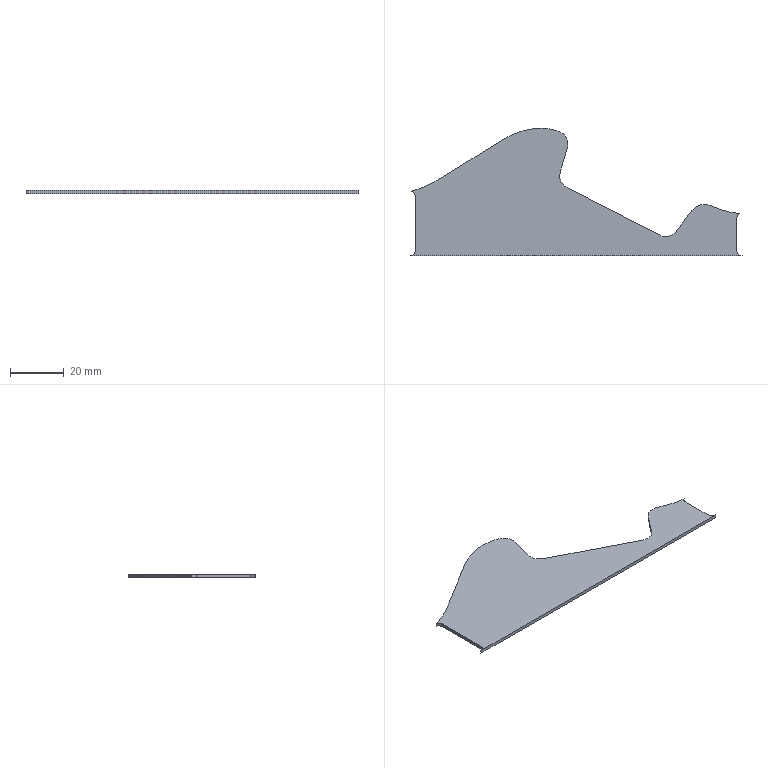Part | STEP file | gslz 2016.10.28-13_id250_x_t | 1 solid | 24 faces | box 124.003 x 47.738 x 1.25 mm | volume 3979 mm3 | plane 12 | cylinder 12 | commonest cylinder face diameters 4 x4 10 x3 12 x1 30 x1 60 x1 66 x1